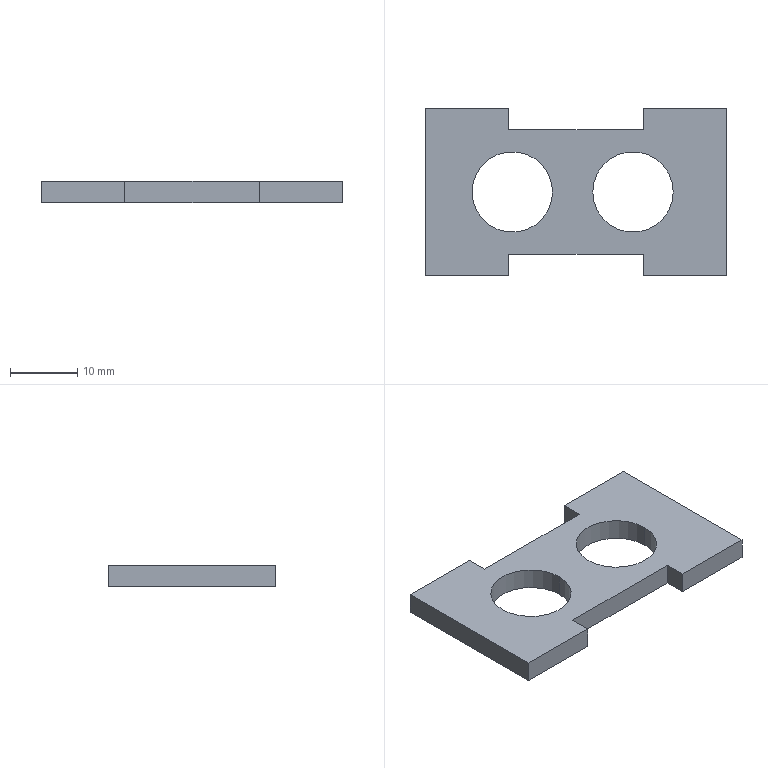Part | SolidWorks | features FlatPattern 1, SMBaseFlange 1, SheetMetal 1 | 1 solid | 18 faces | box 45 x 25 x 3.2 mm | volume 2467 mm3 | plane 14 | cylinder 4 | commonest cylinder face diameters 12 x4
STEP:
#1=CARTESIAN_POINT('',(25.,-9.3,3.2));
#2=VERTEX_POINT('',#1);
#3=CARTESIAN_POINT('',(37.,-9.3,3.2));
#4=VERTEX_POINT('',#3);
#5=CARTESIAN_POINT('',(31.,-9.3,3.2));
#6=DIRECTION('',(0.,0.,1.));
#7=DIRECTION('',(1.,0.,0.));
#8=AXIS2_PLACEMENT_3D('',#5,#6,#7);
#9=CIRCLE('',#8,6.);
#10=EDGE_CURVE('',#2,#4,#9,.T.);
#11=ORIENTED_EDGE('',*,*,#10,.T.);
#12=CARTESIAN_POINT('',(37.,-9.3,0.));
#13=VERTEX_POINT('',#12);
#14=CARTESIAN_POINT('',(37.,-9.3,3.2));
#15=DIRECTION('',(0.,0.,-1.));
#16=VECTOR('',#15,1000.);
#17=LINE('',#14,#16);
#18=EDGE_CURVE('',#4,#13,#17,.T.);
#19=ORIENTED_EDGE('',*,*,#18,.T.);
#20=CARTESIAN_POINT('',(25.,-9.3,0.));
#21=VERTEX_POINT('',#20);
#22=CARTESIAN_POINT('',(31.,-9.3,0.));
#23=DIRECTION('',(0.,0.,1.));
#24=DIRECTION('',(1.,0.,0.));
#25=AXIS2_PLACEMENT_3D('',#22,#23,#24);
#26=CIRCLE('',#25,6.);
#27=EDGE_CURVE('',#21,#13,#26,.T.);
#28=ORIENTED_EDGE('',*,*,#27,.F.);
#29=CARTESIAN_POINT('',(25.,-9.3,3.2));
#30=DIRECTION('',(0.,0.,-1.));
#31=VECTOR('',#30,1000.);
#32=LINE('',#29,#31);
#33=EDGE_CURVE('',#2,#21,#32,.T.);
#34=ORIENTED_EDGE('',*,*,#33,.F.);
#35=EDGE_LOOP('',(#11,#19,#28,#34));
#36=FACE_OUTER_BOUND('',#35,.T.);
#37=CARTESIAN_POINT('',(31.,-9.3,3.2));
#38=DIRECTION('',(0.,0.,-1.));
#39=DIRECTION('',(-1.,0.,0.));
#40=AXIS2_PLACEMENT_3D('',#37,#38,#39);
#41=CYLINDRICAL_SURFACE('',#40,6.);
#42=ADVANCED_FACE('',(#36),#41,.F.);
#43=CARTESIAN_POINT('',(7.,-9.3,3.2));
#44=VERTEX_POINT('',#43);
#45=CARTESIAN_POINT('',(19.,-9.3,3.2));
#46=VERTEX_POINT('',#45);
#47=CARTESIAN_POINT('',(13.,-9.3,3.2));
#48=DIRECTION('',(0.,0.,1.));
#49=DIRECTION('',(1.,0.,0.));
#50=AXIS2_PLACEMENT_3D('',#47,#48,#49);
#51=CIRCLE('',#50,6.);
#52=EDGE_CURVE('',#44,#46,#51,.T.);
#53=ORIENTED_EDGE('',*,*,#52,.T.);
#54=CARTESIAN_POINT('',(19.,-9.3,0.));
#55=VERTEX_POINT('',#54);
#56=CARTESIAN_POINT('',(19.,-9.3,3.2));
#57=DIRECTION('',(0.,0.,-1.));
#58=VECTOR('',#57,1000.);
#59=LINE('',#56,#58);
#60=EDGE_CURVE('',#46,#55,#59,.T.);
#61=ORIENTED_EDGE('',*,*,#60,.T.);
#62=CARTESIAN_POINT('',(7.,-9.3,0.));
#63=VERTEX_POINT('',#62);
#64=CARTESIAN_POINT('',(13.,-9.3,0.));
#65=DIRECTION('',(0.,0.,1.));
#66=DIRECTION('',(1.,0.,0.));
#67=AXIS2_PLACEMENT_3D('',#64,#65,#66);
#68=CIRCLE('',#67,6.);
#69=EDGE_CURVE('',#63,#55,#68,.T.);
#70=ORIENTED_EDGE('',*,*,#69,.F.);
#71=CARTESIAN_POINT('',(7.,-9.3,3.2));
#72=DIRECTION('',(0.,0.,-1.));
#73=VECTOR('',#72,1000.);
#74=LINE('',#71,#73);
#75=EDGE_CURVE('',#44,#63,#74,.T.);
#76=ORIENTED_EDGE('',*,*,#75,.F.);
#77=EDGE_LOOP('',(#53,#61,#70,#76));
#78=FACE_OUTER_BOUND('',#77,.T.);
#79=CARTESIAN_POINT('',(13.,-9.3,3.2));
#80=DIRECTION('',(0.,0.,-1.));
#81=DIRECTION('',(-1.,0.,0.));
#82=AXIS2_PLACEMENT_3D('',#79,#80,#81);
#83=CYLINDRICAL_SURFACE('',#82,6.);
#84=ADVANCED_FACE('',(#78),#83,.F.);
#85=CARTESIAN_POINT('',(0.,3.2,3.2));
#86=VERTEX_POINT('',#85);
#87=CARTESIAN_POINT('',(0.,-21.8,3.2));
#88=VERTEX_POINT('',#87);
#89=CARTESIAN_POINT('',(0.,-21.8,3.2));
#90=DIRECTION('',(0.,-1.,0.));
#91=VECTOR('',#90,1000.);
#92=LINE('',#89,#91);
#93=EDGE_CURVE('',#86,#88,#92,.T.);
#94=ORIENTED_EDGE('',*,*,#93,.T.);
#95=CARTESIAN_POINT('',(12.5,-21.8,3.2));
#96=VERTEX_POINT('',#95);
#97=CARTESIAN_POINT('',(0.,-21.8,3.2));
#98=DIRECTION('',(1.,0.,0.));
#99=VECTOR('',#98,1000.);
#100=LINE('',#97,#99);
#101=EDGE_CURVE('',#88,#96,#100,.T.);
#102=ORIENTED_EDGE('',*,*,#101,.T.);
#103=CARTESIAN_POINT('',(12.5,-18.6,3.2));
#104=VERTEX_POINT('',#103);
#105=CARTESIAN_POINT('',(12.5,-21.8,3.2));
#106=DIRECTION('',(0.,1.,0.));
#107=VECTOR('',#106,1000.);
#108=LINE('',#105,#107);
#109=EDGE_CURVE('',#96,#104,#108,.T.);
#110=ORIENTED_EDGE('',*,*,#109,.T.);
#111=CARTESIAN_POINT('',(32.5,-18.6,3.2));
#112=VERTEX_POINT('',#111);
#113=CARTESIAN_POINT('',(12.5,-18.6,3.2));
#114=DIRECTION('',(1.,0.,0.));
#115=VECTOR('',#114,1000.);
#116=LINE('',#113,#115);
#117=EDGE_CURVE('',#104,#112,#116,.T.);
#118=ORIENTED_EDGE('',*,*,#117,.T.);
#119=CARTESIAN_POINT('',(32.5,-21.8,3.2));
#120=VERTEX_POINT('',#119);
#121=CARTESIAN_POINT('',(32.5,-18.6,3.2));
#122=DIRECTION('',(0.,-1.,0.));
#123=VECTOR('',#122,1000.);
#124=LINE('',#121,#123);
#125=EDGE_CURVE('',#112,#120,#124,.T.);
#126=ORIENTED_EDGE('',*,*,#125,.T.);
#127=CARTESIAN_POINT('',(45.,-21.8,3.2));
#128=VERTEX_POINT('',#127);
#129=CARTESIAN_POINT('',(32.5,-21.8,3.2));
#130=DIRECTION('',(1.,0.,0.));
#131=VECTOR('',#130,1000.);
#132=LINE('',#129,#131);
#133=EDGE_CURVE('',#120,#128,#132,.T.);
#134=ORIENTED_EDGE('',*,*,#133,.T.);
#135=CARTESIAN_POINT('',(45.,3.2,3.2));
#136=VERTEX_POINT('',#135);
#137=CARTESIAN_POINT('',(45.,-21.8,3.2));
#138=DIRECTION('',(0.,1.,0.));
#139=VECTOR('',#138,1000.);
#140=LINE('',#137,#139);
#141=EDGE_CURVE('',#128,#136,#140,.T.);
#142=ORIENTED_EDGE('',*,*,#141,.T.);
#143=CARTESIAN_POINT('',(32.5,3.2,3.2));
#144=VERTEX_POINT('',#143);
#145=CARTESIAN_POINT('',(32.5,3.2,3.2));
#146=DIRECTION('',(-1.,0.,0.));
#147=VECTOR('',#146,1000.);
#148=LINE('',#145,#147);
#149=EDGE_CURVE('',#136,#144,#148,.T.);
#150=ORIENTED_EDGE('',*,*,#149,.T.);
#151=CARTESIAN_POINT('',(32.5,0.,3.2));
#152=VERTEX_POINT('',#151);
#153=CARTESIAN_POINT('',(32.5,0.,3.2));
#154=DIRECTION('',(0.,-1.,0.));
#155=VECTOR('',#154,1000.);
#156=LINE('',#153,#155);
#157=EDGE_CURVE('',#144,#152,#156,.T.);
#158=ORIENTED_EDGE('',*,*,#157,.T.);
#159=CARTESIAN_POINT('',(12.5,0.,3.2));
#160=VERTEX_POINT('',#159);
#161=CARTESIAN_POINT('',(12.5,0.,3.2));
#162=DIRECTION('',(-1.,0.,0.));
#163=VECTOR('',#162,1000.);
#164=LINE('',#161,#163);
#165=EDGE_CURVE('',#152,#160,#164,.T.);
#166=ORIENTED_EDGE('',*,*,#165,.T.);
#167=CARTESIAN_POINT('',(12.5,3.2,3.2));
#168=VERTEX_POINT('',#167);
#169=CARTESIAN_POINT('',(12.5,0.,3.2));
#170=DIRECTION('',(0.,1.,0.));
#171=VECTOR('',#170,1000.);
#172=LINE('',#169,#171);
#173=EDGE_CURVE('',#160,#168,#172,.T.);
#174=ORIENTED_EDGE('',*,*,#173,.T.);
#175=CARTESIAN_POINT('',(0.,3.2,3.2));
#176=DIRECTION('',(-1.,0.,0.));
#177=VECTOR('',#176,1000.);
#178=LINE('',#175,#177);
#179=EDGE_CURVE('',#168,#86,#178,.T.);
#180=ORIENTED_EDGE('',*,*,#179,.T.);
#181=EDGE_LOOP('',(#94,#102,#110,#118,#126,#134,#142,#150,#158,#166,#174,#180));
#182=FACE_OUTER_BOUND('',#181,.T.);
#183=ORIENTED_EDGE('',*,*,#52,.F.);
#184=CARTESIAN_POINT('',(13.,-9.3,3.2));
#185=DIRECTION('',(0.,0.,1.));
#186=DIRECTION('',(1.,0.,0.));
#187=AXIS2_PLACEMENT_3D('',#184,#185,#186);
#188=CIRCLE('',#187,6.);
#189=EDGE_CURVE('',#46,#44,#188,.T.);
#190=ORIENTED_EDGE('',*,*,#189,.F.);
#191=EDGE_LOOP('',(#183,#190));
#192=FACE_BOUND('',#191,.T.);
#193=ORIENTED_EDGE('',*,*,#10,.F.);
#194=CARTESIAN_POINT('',(31.,-9.3,3.2));
#195=DIRECTION('',(0.,0.,1.));
#196=DIRECTION('',(1.,0.,0.));
#197=AXIS2_PLACEMENT_3D('',#194,#195,#196);
#198=CIRCLE('',#197,6.);
#199=EDGE_CURVE('',#4,#2,#198,.T.);
#200=ORIENTED_EDGE('',*,*,#199,.F.);
#201=EDGE_LOOP('',(#193,#200));
#202=FACE_BOUND('',#201,.T.);
#203=CARTESIAN_POINT('',(0.,0.,3.2));
#204=DIRECTION('',(0.,0.,-1.));
#205=DIRECTION('',(-1.,0.,0.));
#206=AXIS2_PLACEMENT_3D('',#203,#204,#205);
#207=PLANE('',#206);
#208=ADVANCED_FACE('',(#182,#192,#202),#207,.F.);
#209=ORIENTED_EDGE('',*,*,#69,.T.);
#210=CARTESIAN_POINT('',(13.,-9.3,0.));
#211=DIRECTION('',(0.,0.,1.));
#212=DIRECTION('',(1.,0.,0.));
#213=AXIS2_PLACEMENT_3D('',#210,#211,#212);
#214=CIRCLE('',#213,6.);
#215=EDGE_CURVE('',#55,#63,#214,.T.);
#216=ORIENTED_EDGE('',*,*,#215,.T.);
#217=EDGE_LOOP('',(#209,#216));
#218=FACE_BOUND('',#217,.T.);
#219=CARTESIAN_POINT('',(0.,3.2,0.));
#220=VERTEX_POINT('',#219);
#221=CARTESIAN_POINT('',(0.,-21.8,0.));
#222=VERTEX_POINT('',#221);
#223=CARTESIAN_POINT('',(0.,-21.8,0.));
#224=DIRECTION('',(0.,-1.,0.));
#225=VECTOR('',#224,1000.);
#226=LINE('',#223,#225);
#227=EDGE_CURVE('',#220,#222,#226,.T.);
#228=ORIENTED_EDGE('',*,*,#227,.F.);
#229=CARTESIAN_POINT('',(12.5,3.2,0.));
#230=VERTEX_POINT('',#229);
#231=CARTESIAN_POINT('',(0.,3.2,0.));
#232=DIRECTION('',(-1.,0.,0.));
#233=VECTOR('',#232,1000.);
#234=LINE('',#231,#233);
#235=EDGE_CURVE('',#230,#220,#234,.T.);
#236=ORIENTED_EDGE('',*,*,#235,.F.);
#237=CARTESIAN_POINT('',(12.5,0.,0.));
#238=VERTEX_POINT('',#237);
#239=CARTESIAN_POINT('',(12.5,0.,0.));
#240=DIRECTION('',(0.,1.,0.));
#241=VECTOR('',#240,1000.);
#242=LINE('',#239,#241);
#243=EDGE_CURVE('',#238,#230,#242,.T.);
#244=ORIENTED_EDGE('',*,*,#243,.F.);
#245=CARTESIAN_POINT('',(32.5,0.,0.));
#246=VERTEX_POINT('',#245);
#247=CARTESIAN_POINT('',(12.5,0.,0.));
#248=DIRECTION('',(-1.,0.,0.));
#249=VECTOR('',#248,1000.);
#250=LINE('',#247,#249);
#251=EDGE_CURVE('',#246,#238,#250,.T.);
#252=ORIENTED_EDGE('',*,*,#251,.F.);
#253=CARTESIAN_POINT('',(32.5,3.2,0.));
#254=VERTEX_POINT('',#253);
#255=CARTESIAN_POINT('',(32.5,0.,0.));
#256=DIRECTION('',(0.,-1.,0.));
#257=VECTOR('',#256,1000.);
#258=LINE('',#255,#257);
#259=EDGE_CURVE('',#254,#246,#258,.T.);
#260=ORIENTED_EDGE('',*,*,#259,.F.);
#261=CARTESIAN_POINT('',(45.,3.2,0.));
#262=VERTEX_POINT('',#261);
#263=CARTESIAN_POINT('',(32.5,3.2,0.));
#264=DIRECTION('',(-1.,0.,0.));
#265=VECTOR('',#264,1000.);
#266=LINE('',#263,#265);
#267=EDGE_CURVE('',#262,#254,#266,.T.);
#268=ORIENTED_EDGE('',*,*,#267,.F.);
#269=CARTESIAN_POINT('',(45.,-21.8,0.));
#270=VERTEX_POINT('',#269);
#271=CARTESIAN_POINT('',(45.,-21.8,0.));
#272=DIRECTION('',(0.,1.,0.));
#273=VECTOR('',#272,1000.);
#274=LINE('',#271,#273);
#275=EDGE_CURVE('',#270,#262,#274,.T.);
#276=ORIENTED_EDGE('',*,*,#275,.F.);
#277=CARTESIAN_POINT('',(32.5,-21.8,0.));
#278=VERTEX_POINT('',#277);
#279=CARTESIAN_POINT('',(32.5,-21.8,0.));
#280=DIRECTION('',(1.,0.,0.));
#281=VECTOR('',#280,1000.);
#282=LINE('',#279,#281);
#283=EDGE_CURVE('',#278,#270,#282,.T.);
#284=ORIENTED_EDGE('',*,*,#283,.F.);
#285=CARTESIAN_POINT('',(32.5,-18.6,0.));
#286=VERTEX_POINT('',#285);
#287=CARTESIAN_POINT('',(32.5,-18.6,0.));
#288=DIRECTION('',(0.,-1.,0.));
#289=VECTOR('',#288,1000.);
#290=LINE('',#287,#289);
#291=EDGE_CURVE('',#286,#278,#290,.T.);
#292=ORIENTED_EDGE('',*,*,#291,.F.);
#293=CARTESIAN_POINT('',(12.5,-18.6,0.));
#294=VERTEX_POINT('',#293);
#295=CARTESIAN_POINT('',(12.5,-18.6,0.));
#296=DIRECTION('',(1.,0.,0.));
#297=VECTOR('',#296,1000.);
#298=LINE('',#295,#297);
#299=EDGE_CURVE('',#294,#286,#298,.T.);
#300=ORIENTED_EDGE('',*,*,#299,.F.);
#301=CARTESIAN_POINT('',(12.5,-21.8,0.));
#302=VERTEX_POINT('',#301);
#303=CARTESIAN_POINT('',(12.5,-21.8,0.));
#304=DIRECTION('',(0.,1.,0.));
#305=VECTOR('',#304,1000.);
#306=LINE('',#303,#305);
#307=EDGE_CURVE('',#302,#294,#306,.T.);
#308=ORIENTED_EDGE('',*,*,#307,.F.);
#309=CARTESIAN_POINT('',(0.,-21.8,0.));
#310=DIRECTION('',(1.,0.,0.));
#311=VECTOR('',#310,1000.);
#312=LINE('',#309,#311);
#313=EDGE_CURVE('',#222,#302,#312,.T.);
#314=ORIENTED_EDGE('',*,*,#313,.F.);
#315=EDGE_LOOP('',(#228,#236,#244,#252,#260,#268,#276,#284,#292,#300,#308,#314));
#316=FACE_OUTER_BOUND('',#315,.T.);
#317=ORIENTED_EDGE('',*,*,#27,.T.);
#318=CARTESIAN_POINT('',(31.,-9.3,0.));
#319=DIRECTION('',(0.,0.,1.));
#320=DIRECTION('',(1.,0.,0.));
#321=AXIS2_PLACEMENT_3D('',#318,#319,#320);
#322=CIRCLE('',#321,6.);
#323=EDGE_CURVE('',#13,#21,#322,.T.);
#324=ORIENTED_EDGE('',*,*,#323,.T.);
#325=EDGE_LOOP('',(#317,#324));
#326=FACE_BOUND('',#325,.T.);
#327=CARTESIAN_POINT('',(0.,0.,0.));
#328=DIRECTION('',(0.,0.,-1.));
#329=DIRECTION('',(-1.,0.,0.));
#330=AXIS2_PLACEMENT_3D('',#327,#328,#329);
#331=PLANE('',#330);
#332=ADVANCED_FACE('',(#218,#316,#326),#331,.T.);
#333=ORIENTED_EDGE('',*,*,#227,.T.);
#334=CARTESIAN_POINT('',(0.,-21.8,3.2));
#335=DIRECTION('',(0.,0.,-1.));
#336=VECTOR('',#335,1000.);
#337=LINE('',#334,#336);
#338=EDGE_CURVE('',#88,#222,#337,.T.);
#339=ORIENTED_EDGE('',*,*,#338,.F.);
#340=ORIENTED_EDGE('',*,*,#93,.F.);
#341=CARTESIAN_POINT('',(0.,3.2,3.2));
#342=DIRECTION('',(0.,0.,-1.));
#343=VECTOR('',#342,1000.);
#344=LINE('',#341,#343);
#345=EDGE_CURVE('',#86,#220,#344,.T.);
#346=ORIENTED_EDGE('',*,*,#345,.T.);
#347=EDGE_LOOP('',(#333,#339,#340,#346));
#348=FACE_OUTER_BOUND('',#347,.T.);
#349=CARTESIAN_POINT('',(0.,-21.8,3.2));
#350=DIRECTION('',(1.,0.,0.));
#351=DIRECTION('',(0.,1.,0.));
#352=AXIS2_PLACEMENT_3D('',#349,#350,#351);
#353=PLANE('',#352);
#354=ADVANCED_FACE('',(#348),#353,.F.);
#355=ORIENTED_EDGE('',*,*,#313,.T.);
#356=CARTESIAN_POINT('',(12.5,-21.8,3.2));
#357=DIRECTION('',(0.,0.,-1.));
#358=VECTOR('',#357,1000.);
#359=LINE('',#356,#358);
#360=EDGE_CURVE('',#96,#302,#359,.T.);
#361=ORIENTED_EDGE('',*,*,#360,.F.);
#362=ORIENTED_EDGE('',*,*,#101,.F.);
#363=ORIENTED_EDGE('',*,*,#338,.T.);
#364=EDGE_LOOP('',(#355,#361,#362,#363));
#365=FACE_OUTER_BOUND('',#364,.T.);
#366=CARTESIAN_POINT('',(0.,-21.8,3.2));
#367=DIRECTION('',(0.,1.,0.));
#368=DIRECTION('',(0.,0.,1.));
#369=AXIS2_PLACEMENT_3D('',#366,#367,#368);
#370=PLANE('',#369);
#371=ADVANCED_FACE('',(#365),#370,.F.);
#372=ORIENTED_EDGE('',*,*,#307,.T.);
#373=CARTESIAN_POINT('',(12.5,-18.6,3.2));
#374=DIRECTION('',(0.,0.,-1.));
#375=VECTOR('',#374,1000.);
#376=LINE('',#373,#375);
#377=EDGE_CURVE('',#104,#294,#376,.T.);
#378=ORIENTED_EDGE('',*,*,#377,.F.);
#379=ORIENTED_EDGE('',*,*,#109,.F.);
#380=ORIENTED_EDGE('',*,*,#360,.T.);
#381=EDGE_LOOP('',(#372,#378,#379,#380));
#382=FACE_OUTER_BOUND('',#381,.T.);
#383=CARTESIAN_POINT('',(12.5,-21.8,3.2));
#384=DIRECTION('',(-1.,0.,0.));
#385=DIRECTION('',(0.,0.,1.));
#386=AXIS2_PLACEMENT_3D('',#383,#384,#385);
#387=PLANE('',#386);
#388=ADVANCED_FACE('',(#382),#387,.F.);
#389=ORIENTED_EDGE('',*,*,#299,.T.);
#390=CARTESIAN_POINT('',(32.5,-18.6,3.2));
#391=DIRECTION('',(0.,0.,-1.));
#392=VECTOR('',#391,1000.);
#393=LINE('',#390,#392);
#394=EDGE_CURVE('',#112,#286,#393,.T.);
#395=ORIENTED_EDGE('',*,*,#394,.F.);
#396=ORIENTED_EDGE('',*,*,#117,.F.);
#397=ORIENTED_EDGE('',*,*,#377,.T.);
#398=EDGE_LOOP('',(#389,#395,#396,#397));
#399=FACE_OUTER_BOUND('',#398,.T.);
#400=CARTESIAN_POINT('',(12.5,-18.6,3.2));
#401=DIRECTION('',(0.,1.,0.));
#402=DIRECTION('',(-1.,0.,0.));
#403=AXIS2_PLACEMENT_3D('',#400,#401,#402);
#404=PLANE('',#403);
#405=ADVANCED_FACE('',(#399),#404,.F.);
#406=ORIENTED_EDGE('',*,*,#291,.T.);
#407=CARTESIAN_POINT('',(32.5,-21.8,3.2));
#408=DIRECTION('',(0.,0.,-1.));
#409=VECTOR('',#408,1000.);
#410=LINE('',#407,#409);
#411=EDGE_CURVE('',#120,#278,#410,.T.);
#412=ORIENTED_EDGE('',*,*,#411,.F.);
#413=ORIENTED_EDGE('',*,*,#125,.F.);
#414=ORIENTED_EDGE('',*,*,#394,.T.);
#415=EDGE_LOOP('',(#406,#412,#413,#414));
#416=FACE_OUTER_BOUND('',#415,.T.);
#417=CARTESIAN_POINT('',(32.5,-18.6,3.2));
#418=DIRECTION('',(1.,0.,0.));
#419=DIRECTION('',(0.,0.,-1.));
#420=AXIS2_PLACEMENT_3D('',#417,#418,#419);
#421=PLANE('',#420);
#422=ADVANCED_FACE('',(#416),#421,.F.);
#423=ORIENTED_EDGE('',*,*,#283,.T.);
#424=CARTESIAN_POINT('',(45.,-21.8,3.2));
#425=DIRECTION('',(0.,0.,-1.));
#426=VECTOR('',#425,1000.);
#427=LINE('',#424,#426);
#428=EDGE_CURVE('',#128,#270,#427,.T.);
#429=ORIENTED_EDGE('',*,*,#428,.F.);
#430=ORIENTED_EDGE('',*,*,#133,.F.);
#431=ORIENTED_EDGE('',*,*,#411,.T.);
#432=EDGE_LOOP('',(#423,#429,#430,#431));
#433=FACE_OUTER_BOUND('',#432,.T.);
#434=CARTESIAN_POINT('',(32.5,-21.8,3.2));
#435=DIRECTION('',(0.,1.,0.));
#436=DIRECTION('',(0.,0.,1.));
#437=AXIS2_PLACEMENT_3D('',#434,#435,#436);
#438=PLANE('',#437);
#439=ADVANCED_FACE('',(#433),#438,.F.);
#440=ORIENTED_EDGE('',*,*,#275,.T.);
#441=CARTESIAN_POINT('',(45.,3.2,3.2));
#442=DIRECTION('',(0.,0.,-1.));
#443=VECTOR('',#442,1000.);
#444=LINE('',#441,#443);
#445=EDGE_CURVE('',#136,#262,#444,.T.);
#446=ORIENTED_EDGE('',*,*,#445,.F.);
#447=ORIENTED_EDGE('',*,*,#141,.F.);
#448=ORIENTED_EDGE('',*,*,#428,.T.);
#449=EDGE_LOOP('',(#440,#446,#447,#448));
#450=FACE_OUTER_BOUND('',#449,.T.);
#451=CARTESIAN_POINT('',(45.,-21.8,3.2));
#452=DIRECTION('',(-1.,0.,0.));
#453=DIRECTION('',(0.,0.,1.));
#454=AXIS2_PLACEMENT_3D('',#451,#452,#453);
#455=PLANE('',#454);
#456=ADVANCED_FACE('',(#450),#455,.F.);
#457=ORIENTED_EDGE('',*,*,#267,.T.);
#458=CARTESIAN_POINT('',(32.5,3.2,3.2));
#459=DIRECTION('',(0.,0.,-1.));
#460=VECTOR('',#459,1000.);
#461=LINE('',#458,#460);
#462=EDGE_CURVE('',#144,#254,#461,.T.);
#463=ORIENTED_EDGE('',*,*,#462,.F.);
#464=ORIENTED_EDGE('',*,*,#149,.F.);
#465=ORIENTED_EDGE('',*,*,#445,.T.);
#466=EDGE_LOOP('',(#457,#463,#464,#465));
#467=FACE_OUTER_BOUND('',#466,.T.);
#468=CARTESIAN_POINT('',(32.5,3.2,3.2));
#469=DIRECTION('',(0.,-1.,0.));
#470=DIRECTION('',(0.,0.,-1.));
#471=AXIS2_PLACEMENT_3D('',#468,#469,#470);
#472=PLANE('',#471);
#473=ADVANCED_FACE('',(#467),#472,.F.);
#474=ORIENTED_EDGE('',*,*,#259,.T.);
#475=CARTESIAN_POINT('',(32.5,0.,3.2));
#476=DIRECTION('',(0.,0.,-1.));
#477=VECTOR('',#476,1000.);
#478=LINE('',#475,#477);
#479=EDGE_CURVE('',#152,#246,#478,.T.);
#480=ORIENTED_EDGE('',*,*,#479,.F.);
#481=ORIENTED_EDGE('',*,*,#157,.F.);
#482=ORIENTED_EDGE('',*,*,#462,.T.);
#483=EDGE_LOOP('',(#474,#480,#481,#482));
#484=FACE_OUTER_BOUND('',#483,.T.);
#485=CARTESIAN_POINT('',(32.5,0.,3.2));
#486=DIRECTION('',(1.,0.,0.));
#487=DIRECTION('',(0.,0.,-1.));
#488=AXIS2_PLACEMENT_3D('',#485,#486,#487);
#489=PLANE('',#488);
#490=ADVANCED_FACE('',(#484),#489,.F.);
#491=ORIENTED_EDGE('',*,*,#251,.T.);
#492=CARTESIAN_POINT('',(12.5,0.,3.2));
#493=DIRECTION('',(0.,0.,-1.));
#494=VECTOR('',#493,1000.);
#495=LINE('',#492,#494);
#496=EDGE_CURVE('',#160,#238,#495,.T.);
#497=ORIENTED_EDGE('',*,*,#496,.F.);
#498=ORIENTED_EDGE('',*,*,#165,.F.);
#499=ORIENTED_EDGE('',*,*,#479,.T.);
#500=EDGE_LOOP('',(#491,#497,#498,#499));
#501=FACE_OUTER_BOUND('',#500,.T.);
#502=CARTESIAN_POINT('',(12.5,0.,3.2));
#503=DIRECTION('',(0.,-1.,0.));
#504=DIRECTION('',(1.,0.,0.));
#505=AXIS2_PLACEMENT_3D('',#502,#503,#504);
#506=PLANE('',#505);
#507=ADVANCED_FACE('',(#501),#506,.F.);
#508=ORIENTED_EDGE('',*,*,#243,.T.);
#509=CARTESIAN_POINT('',(12.5,3.2,3.2));
#510=DIRECTION('',(0.,0.,-1.));
#511=VECTOR('',#510,1000.);
#512=LINE('',#509,#511);
#513=EDGE_CURVE('',#168,#230,#512,.T.);
#514=ORIENTED_EDGE('',*,*,#513,.F.);
#515=ORIENTED_EDGE('',*,*,#173,.F.);
#516=ORIENTED_EDGE('',*,*,#496,.T.);
#517=EDGE_LOOP('',(#508,#514,#515,#516));
#518=FACE_OUTER_BOUND('',#517,.T.);
#519=CARTESIAN_POINT('',(12.5,0.,3.2));
#520=DIRECTION('',(-1.,0.,0.));
#521=DIRECTION('',(0.,0.,1.));
#522=AXIS2_PLACEMENT_3D('',#519,#520,#521);
#523=PLANE('',#522);
#524=ADVANCED_FACE('',(#518),#523,.F.);
#525=ORIENTED_EDGE('',*,*,#235,.T.);
#526=ORIENTED_EDGE('',*,*,#345,.F.);
#527=ORIENTED_EDGE('',*,*,#179,.F.);
#528=ORIENTED_EDGE('',*,*,#513,.T.);
#529=EDGE_LOOP('',(#525,#526,#527,#528));
#530=FACE_OUTER_BOUND('',#529,.T.);
#531=CARTESIAN_POINT('',(0.,3.2,3.2));
#532=DIRECTION('',(0.,-1.,0.));
#533=DIRECTION('',(1.,0.,0.));
#534=AXIS2_PLACEMENT_3D('',#531,#532,#533);
#535=PLANE('',#534);
#536=ADVANCED_FACE('',(#530),#535,.F.);
#537=ORIENTED_EDGE('',*,*,#60,.F.);
#538=ORIENTED_EDGE('',*,*,#189,.T.);
#539=ORIENTED_EDGE('',*,*,#75,.T.);
#540=ORIENTED_EDGE('',*,*,#215,.F.);
#541=EDGE_LOOP('',(#537,#538,#539,#540));
#542=FACE_OUTER_BOUND('',#541,.T.);
#543=CARTESIAN_POINT('',(13.,-9.3,3.2));
#544=DIRECTION('',(0.,0.,-1.));
#545=DIRECTION('',(-1.,0.,0.));
#546=AXIS2_PLACEMENT_3D('',#543,#544,#545);
#547=CYLINDRICAL_SURFACE('',#546,6.);
#548=ADVANCED_FACE('',(#542),#547,.F.);
#549=ORIENTED_EDGE('',*,*,#18,.F.);
#550=ORIENTED_EDGE('',*,*,#199,.T.);
#551=ORIENTED_EDGE('',*,*,#33,.T.);
#552=ORIENTED_EDGE('',*,*,#323,.F.);
#553=EDGE_LOOP('',(#549,#550,#551,#552));
#554=FACE_OUTER_BOUND('',#553,.T.);
#555=CARTESIAN_POINT('',(31.,-9.3,3.2));
#556=DIRECTION('',(0.,0.,-1.));
#557=DIRECTION('',(-1.,0.,0.));
#558=AXIS2_PLACEMENT_3D('',#555,#556,#557);
#559=CYLINDRICAL_SURFACE('',#558,6.);
#560=ADVANCED_FACE('',(#554),#559,.F.);
#561=CLOSED_SHELL('',(#42,#84,#208,#332,#354,#371,#388,#405,#422,#439,#456,#473,#490,#507,#524,#536,#548,#560));
#562=MANIFOLD_SOLID_BREP('',#561);
#563=CARTESIAN_POINT('',(0.,0.,0.));
#564=DIRECTION('',(0.,0.,1.));
#565=DIRECTION('',(1.,0.,0.));
#566=AXIS2_PLACEMENT_3D('',#563,#564,#565);
#567=(LENGTH_UNIT()NAMED_UNIT(*)SI_UNIT(.MILLI.,.METRE.));
#568=UNCERTAINTY_MEASURE_WITH_UNIT(LENGTH_MEASURE(0.00001),#567,'','');
#569=(NAMED_UNIT(*)PLANE_ANGLE_UNIT()SI_UNIT($,.RADIAN.));
#570=(NAMED_UNIT(*)SI_UNIT($,.STERADIAN.)SOLID_ANGLE_UNIT());
#571=(GEOMETRIC_REPRESENTATION_CONTEXT(3)GLOBAL_UNCERTAINTY_ASSIGNED_CONTEXT((#568))GLOBAL_UNIT_ASSIGNED_CONTEXT((#567,#569,#570))REPRESENTATION_CONTEXT('',''));
#572=ADVANCED_BREP_SHAPE_REPRESENTATION('',(#562,#566),#571);